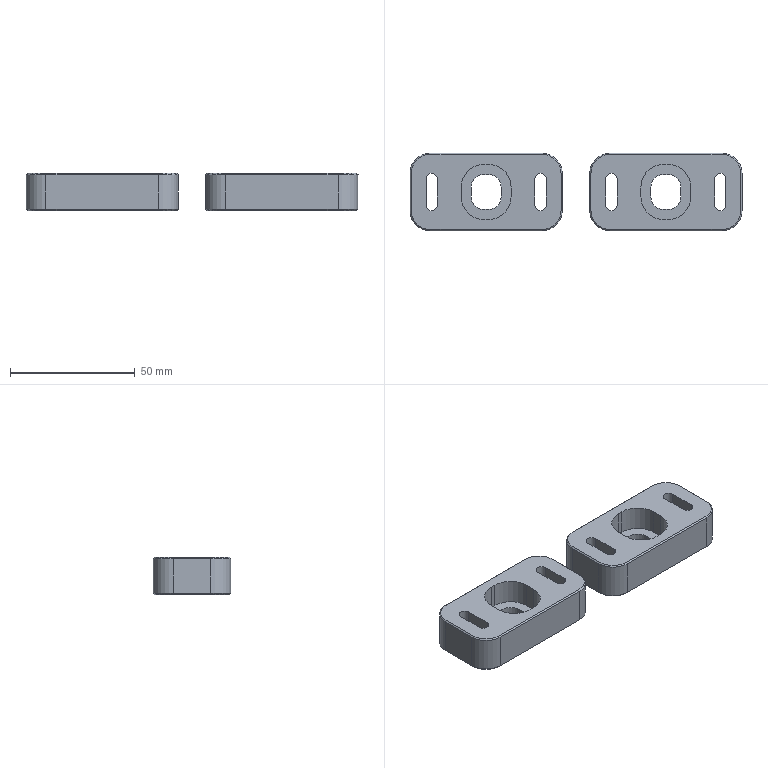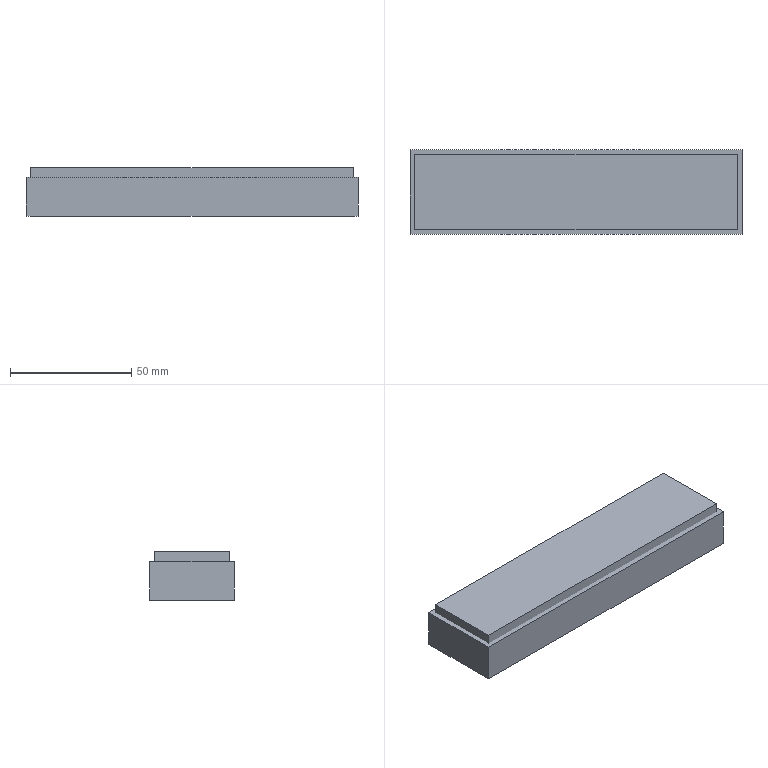CAM job | NX | 3-axis milling | part box 133 x 31 x 15 mm | stock box 137 x 35 x 20 mm
Tools:
number,name,description,diameter,corner_radius,flute_length,length,flutes
1,D63,Milling Tool-5 Parameters,63.0,0.0,50.0,75.0,2
9,D10,Milling Tool-5 Parameters,10.0,0.0,50.0,75.0,2
2,D4A45,Milling Tool-5 Parameters,4.0,0.0,2.0,2.0,2
10,D10JING,Milling Tool-5 Parameters,10.0,0.0,50.0,75.0,2
4,D4,Milling Tool-5 Parameters,4.0,0.0,50.0,75.0,2
Operations:
program,operation,operation_type,tool,method,geometry_group,spindle_rpm,surface_speed,feed_per_tooth,feed_cut,feed_plunge,cut_length_mm,path_length_mm,cut_time_min,machine_time_min
1虎钳,FLOOR_WALL,VolumeBased25DMillingOperation,D63,METHOD,A,6500.0,1286.0,0.0962,1250.0,100.0,212.0,266.0,0.1696,0.175
1虎钳,ZLEVEL_PROFILE_1_COPY_1_COPY,ZLevelMilling,D4A45,METHOD,A,9500.0,179.0,0.0526,1000.0,100.0,621.456,1389.718,0.6215,0.6983
1虎钳,ZLEVEL_PROFILE,ZLevelMilling,D10,METHOD,A,9500.0,298.0,0.1579,3000.0,1000.0,6282.632,6570.154,2.158,2.187
1虎钳,ZLEVEL_PROFILE_COPY,ZLevelMilling,D10,METHOD,A,9500.0,298.0,0.1579,3000.0,1000.0,881.651,1087.678,0.3576,0.3782
1虎钳,ZLEVEL_PROFILE_COPY_COPY_1,ZLevelMilling,D10,METHOD,A,9500.0,298.0,0.1579,3000.0,1000.0,227.006,463.281,0.1394,0.163
1虎钳,ZLEVEL_PROFILE_COPY_COPY,ZLevelMilling,D10JING,MILL_FINISH,A,9500.0,119.0,0.0632,1200.0,1000.0,452.135,977.795,0.3788,0.4314
1虎钳,ZLEVEL_PROFILE_COPY_COPY_COPY,ZLevelMilling,D10JING,MILL_FINISH,A,9500.0,119.0,0.0632,1200.0,1000.0,87.489,310.999,0.0741,0.0964
1虎钳,ZLEVEL_PROFILE_COPY_COPY_1_COPY,ZLevelMilling,D4,METHOD,A,9500.0,119.0,0.0632,1200.0,1000.0,4716.65,5121.045,3.954,3.994
2,FLOOR_WALL_COPY,VolumeBased25DMillingOperation,D63,METHOD,B,6500.0,1286.0,0.0962,1250.0,100.0,1040.0,2098.001,0.832,0.9378
2,ZLEVEL_PROFILE_1_COPY_1_COPY_COPY,ZLevelMilling,D4A45,METHOD,B,9500.0,179.0,0.0526,1000.0,100.0,571.309,1370.889,0.5713,0.6513